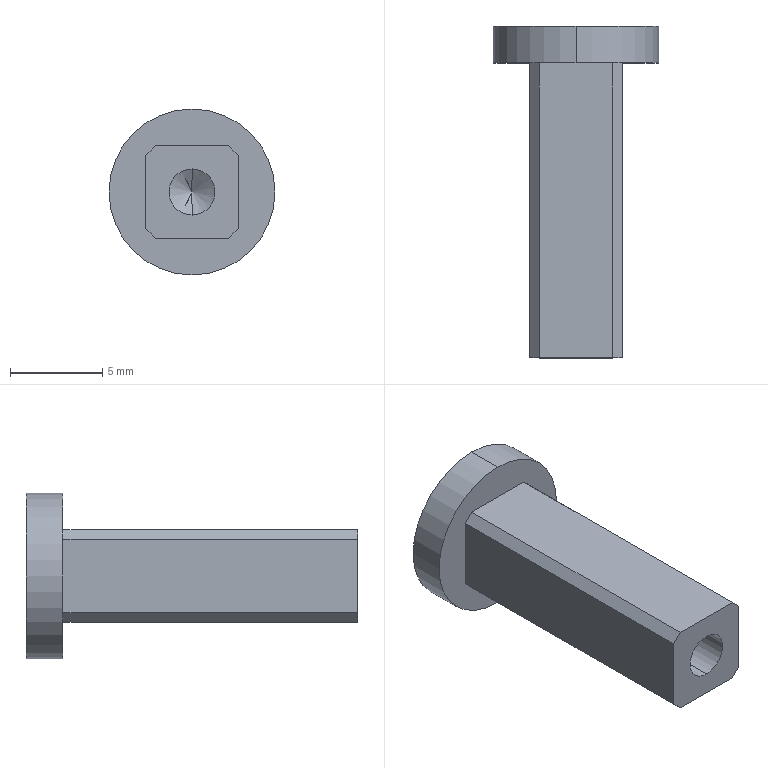Part | SolidWorks | features Chamfer 1, Extrusion 1, HoleWzd 1, ICE 1 | 1 solid | 17 faces | box 9 x 18 x 9 mm | volume 476.281 mm3 | plane 11 | cylinder 4 | cone 2 | commonest cylinder face diameters 2.5 x2 9 x2
STEP:
#1=CARTESIAN_POINT('',(0.,-0.5,1.25));
#2=VERTEX_POINT('',#1);
#3=CARTESIAN_POINT('',(0.,-0.5,-1.25));
#4=VERTEX_POINT('',#3);
#5=CARTESIAN_POINT('',(0.,-0.5,0.));
#6=DIRECTION('',(0.,-1.,0.));
#7=DIRECTION('',(0.,0.,-1.));
#8=AXIS2_PLACEMENT_3D('',#5,#6,#7);
#9=CIRCLE('',#8,1.25);
#10=EDGE_CURVE('',#2,#4,#9,.T.);
#11=ORIENTED_EDGE('',*,*,#10,.F.);
#12=CARTESIAN_POINT('',(0.,-9.,1.25));
#13=VERTEX_POINT('',#12);
#14=CARTESIAN_POINT('',(0.,-9.,1.25));
#15=DIRECTION('',(0.,-1.,0.));
#16=VECTOR('',#15,1000.);
#17=LINE('',#14,#16);
#18=EDGE_CURVE('',#2,#13,#17,.T.);
#19=ORIENTED_EDGE('',*,*,#18,.T.);
#20=CARTESIAN_POINT('',(0.,-9.,-1.25));
#21=VERTEX_POINT('',#20);
#22=CARTESIAN_POINT('',(0.,-9.,0.));
#23=DIRECTION('',(0.,-1.,0.));
#24=DIRECTION('',(0.,0.,-1.));
#25=AXIS2_PLACEMENT_3D('',#22,#23,#24);
#26=CIRCLE('',#25,1.25);
#27=EDGE_CURVE('',#13,#21,#26,.T.);
#28=ORIENTED_EDGE('',*,*,#27,.T.);
#29=CARTESIAN_POINT('',(0.,-9.,-1.25));
#30=DIRECTION('',(0.,-1.,0.));
#31=VECTOR('',#30,1000.);
#32=LINE('',#29,#31);
#33=EDGE_CURVE('',#4,#21,#32,.T.);
#34=ORIENTED_EDGE('',*,*,#33,.F.);
#35=EDGE_LOOP('',(#11,#19,#28,#34));
#36=FACE_OUTER_BOUND('',#35,.T.);
#37=CARTESIAN_POINT('',(0.,-9.,0.));
#38=DIRECTION('',(0.,-1.,0.));
#39=DIRECTION('',(0.,0.,-1.));
#40=AXIS2_PLACEMENT_3D('',#37,#38,#39);
#41=CYLINDRICAL_SURFACE('',#40,1.25);
#42=ADVANCED_FACE('',(#36),#41,.F.);
#43=CARTESIAN_POINT('',(0.,0.2511,0.));
#44=VERTEX_POINT('',#43);
#45=CARTESIAN_POINT('',(0.,-0.5,-1.25));
#46=DIRECTION('',(0.,-0.515,-0.8572));
#47=VECTOR('',#46,1000.);
#48=LINE('',#45,#47);
#49=EDGE_CURVE('',#44,#4,#48,.T.);
#50=ORIENTED_EDGE('',*,*,#49,.F.);
#51=CARTESIAN_POINT('',(0.,-0.5,1.25));
#52=DIRECTION('',(0.,-0.515,0.8572));
#53=VECTOR('',#52,1000.);
#54=LINE('',#51,#53);
#55=EDGE_CURVE('',#44,#2,#54,.T.);
#56=ORIENTED_EDGE('',*,*,#55,.T.);
#57=ORIENTED_EDGE('',*,*,#10,.T.);
#58=EDGE_LOOP('',(#50,#56,#57));
#59=FACE_OUTER_BOUND('',#58,.T.);
#60=CARTESIAN_POINT('',(0.,-0.5,0.));
#61=DIRECTION('',(0.,-1.,0.));
#62=DIRECTION('',(0.,0.,-1.));
#63=AXIS2_PLACEMENT_3D('',#60,#61,#62);
#64=CONICAL_SURFACE('',#63,1.25,1.03);
#65=ADVANCED_FACE('',(#59),#64,.F.);
#66=CARTESIAN_POINT('',(0.,9.,4.5));
#67=VERTEX_POINT('',#66);
#68=CARTESIAN_POINT('',(0.,9.,-4.5));
#69=VERTEX_POINT('',#68);
#70=CARTESIAN_POINT('',(0.,9.,0.));
#71=DIRECTION('',(0.,1.,0.));
#72=DIRECTION('',(0.,0.,1.));
#73=AXIS2_PLACEMENT_3D('',#70,#71,#72);
#74=CIRCLE('',#73,4.5);
#75=EDGE_CURVE('',#67,#69,#74,.T.);
#76=ORIENTED_EDGE('',*,*,#75,.F.);
#77=CARTESIAN_POINT('',(0.,7.,4.5));
#78=VERTEX_POINT('',#77);
#79=CARTESIAN_POINT('',(0.,9.,4.5));
#80=DIRECTION('',(0.,-1.,0.));
#81=VECTOR('',#80,1000.);
#82=LINE('',#79,#81);
#83=EDGE_CURVE('',#67,#78,#82,.T.);
#84=ORIENTED_EDGE('',*,*,#83,.T.);
#85=CARTESIAN_POINT('',(0.,7.,-4.5));
#86=VERTEX_POINT('',#85);
#87=CARTESIAN_POINT('',(0.,7.,0.));
#88=DIRECTION('',(0.,-1.,0.));
#89=DIRECTION('',(0.,0.,-1.));
#90=AXIS2_PLACEMENT_3D('',#87,#88,#89);
#91=CIRCLE('',#90,4.5);
#92=EDGE_CURVE('',#86,#78,#91,.T.);
#93=ORIENTED_EDGE('',*,*,#92,.F.);
#94=CARTESIAN_POINT('',(0.,9.,-4.5));
#95=DIRECTION('',(0.,-1.,0.));
#96=VECTOR('',#95,1000.);
#97=LINE('',#94,#96);
#98=EDGE_CURVE('',#69,#86,#97,.T.);
#99=ORIENTED_EDGE('',*,*,#98,.F.);
#100=EDGE_LOOP('',(#76,#84,#93,#99));
#101=FACE_OUTER_BOUND('',#100,.T.);
#102=CARTESIAN_POINT('',(0.,9.,0.));
#103=DIRECTION('',(0.,-1.,0.));
#104=DIRECTION('',(0.,0.,-1.));
#105=AXIS2_PLACEMENT_3D('',#102,#103,#104);
#106=CYLINDRICAL_SURFACE('',#105,4.5);
#107=ADVANCED_FACE('',(#101),#106,.T.);
#108=ORIENTED_EDGE('',*,*,#83,.F.);
#109=CARTESIAN_POINT('',(0.,9.,0.));
#110=DIRECTION('',(0.,1.,0.));
#111=DIRECTION('',(0.,0.,1.));
#112=AXIS2_PLACEMENT_3D('',#109,#110,#111);
#113=CIRCLE('',#112,4.5);
#114=EDGE_CURVE('',#69,#67,#113,.T.);
#115=ORIENTED_EDGE('',*,*,#114,.F.);
#116=ORIENTED_EDGE('',*,*,#98,.T.);
#117=CARTESIAN_POINT('',(0.,7.,0.));
#118=DIRECTION('',(0.,-1.,0.));
#119=DIRECTION('',(0.,0.,-1.));
#120=AXIS2_PLACEMENT_3D('',#117,#118,#119);
#121=CIRCLE('',#120,4.5);
#122=EDGE_CURVE('',#78,#86,#121,.T.);
#123=ORIENTED_EDGE('',*,*,#122,.F.);
#124=EDGE_LOOP('',(#108,#115,#116,#123));
#125=FACE_OUTER_BOUND('',#124,.T.);
#126=CARTESIAN_POINT('',(0.,9.,0.));
#127=DIRECTION('',(0.,-1.,0.));
#128=DIRECTION('',(0.,0.,-1.));
#129=AXIS2_PLACEMENT_3D('',#126,#127,#128);
#130=CYLINDRICAL_SURFACE('',#129,4.5);
#131=ADVANCED_FACE('',(#125),#130,.T.);
#132=ORIENTED_EDGE('',*,*,#114,.T.);
#133=ORIENTED_EDGE('',*,*,#75,.T.);
#134=EDGE_LOOP('',(#132,#133));
#135=FACE_OUTER_BOUND('',#134,.T.);
#136=CARTESIAN_POINT('',(0.,9.,0.));
#137=DIRECTION('',(0.,1.,0.));
#138=DIRECTION('',(0.,0.,1.));
#139=AXIS2_PLACEMENT_3D('',#136,#137,#138);
#140=PLANE('',#139);
#141=ADVANCED_FACE('',(#135),#140,.T.);
#142=CARTESIAN_POINT('',(-2.,7.,-2.5));
#143=VERTEX_POINT('',#142);
#144=CARTESIAN_POINT('',(2.,7.,-2.5));
#145=VERTEX_POINT('',#144);
#146=CARTESIAN_POINT('',(-2.5,7.,-2.5));
#147=DIRECTION('',(1.,0.,0.));
#148=VECTOR('',#147,1000.);
#149=LINE('',#146,#148);
#150=EDGE_CURVE('',#143,#145,#149,.T.);
#151=ORIENTED_EDGE('',*,*,#150,.F.);
#152=CARTESIAN_POINT('',(-2.5,7.,-2.));
#153=VERTEX_POINT('',#152);
#154=CARTESIAN_POINT('',(-2.5,7.,-2.));
#155=DIRECTION('',(-0.7071,0.,0.7071));
#156=VECTOR('',#155,1000.);
#157=LINE('',#154,#156);
#158=EDGE_CURVE('',#143,#153,#157,.T.);
#159=ORIENTED_EDGE('',*,*,#158,.T.);
#160=CARTESIAN_POINT('',(-2.5,7.,2.));
#161=VERTEX_POINT('',#160);
#162=CARTESIAN_POINT('',(-2.5,7.,-2.5));
#163=DIRECTION('',(0.,0.,-1.));
#164=VECTOR('',#163,1000.);
#165=LINE('',#162,#164);
#166=EDGE_CURVE('',#161,#153,#165,.T.);
#167=ORIENTED_EDGE('',*,*,#166,.F.);
#168=CARTESIAN_POINT('',(-2.,7.,2.5));
#169=VERTEX_POINT('',#168);
#170=CARTESIAN_POINT('',(-2.,7.,2.5));
#171=DIRECTION('',(0.7071,0.,0.7071));
#172=VECTOR('',#171,1000.);
#173=LINE('',#170,#172);
#174=EDGE_CURVE('',#161,#169,#173,.T.);
#175=ORIENTED_EDGE('',*,*,#174,.T.);
#176=CARTESIAN_POINT('',(2.,7.,2.5));
#177=VERTEX_POINT('',#176);
#178=CARTESIAN_POINT('',(-2.5,7.,2.5));
#179=DIRECTION('',(-1.,0.,0.));
#180=VECTOR('',#179,1000.);
#181=LINE('',#178,#180);
#182=EDGE_CURVE('',#177,#169,#181,.T.);
#183=ORIENTED_EDGE('',*,*,#182,.F.);
#184=CARTESIAN_POINT('',(2.5,7.,2.));
#185=VERTEX_POINT('',#184);
#186=CARTESIAN_POINT('',(2.5,7.,2.));
#187=DIRECTION('',(0.7071,0.,-0.7071));
#188=VECTOR('',#187,1000.);
#189=LINE('',#186,#188);
#190=EDGE_CURVE('',#177,#185,#189,.T.);
#191=ORIENTED_EDGE('',*,*,#190,.T.);
#192=CARTESIAN_POINT('',(2.5,7.,-2.));
#193=VERTEX_POINT('',#192);
#194=CARTESIAN_POINT('',(2.5,7.,-2.5));
#195=DIRECTION('',(0.,0.,1.));
#196=VECTOR('',#195,1000.);
#197=LINE('',#194,#196);
#198=EDGE_CURVE('',#193,#185,#197,.T.);
#199=ORIENTED_EDGE('',*,*,#198,.F.);
#200=CARTESIAN_POINT('',(2.,7.,-2.5));
#201=DIRECTION('',(-0.7071,0.,-0.7071));
#202=VECTOR('',#201,1000.);
#203=LINE('',#200,#202);
#204=EDGE_CURVE('',#193,#145,#203,.T.);
#205=ORIENTED_EDGE('',*,*,#204,.T.);
#206=EDGE_LOOP('',(#151,#159,#167,#175,#183,#191,#199,#205));
#207=FACE_BOUND('',#206,.T.);
#208=ORIENTED_EDGE('',*,*,#92,.T.);
#209=ORIENTED_EDGE('',*,*,#122,.T.);
#210=EDGE_LOOP('',(#208,#209));
#211=FACE_OUTER_BOUND('',#210,.T.);
#212=CARTESIAN_POINT('',(0.,7.,0.));
#213=DIRECTION('',(0.,-1.,0.));
#214=DIRECTION('',(0.,0.,-1.));
#215=AXIS2_PLACEMENT_3D('',#212,#213,#214);
#216=PLANE('',#215);
#217=ADVANCED_FACE('',(#207,#211),#216,.T.);
#218=CARTESIAN_POINT('',(2.5,-9.,-2.));
#219=VERTEX_POINT('',#218);
#220=CARTESIAN_POINT('',(2.5,-9.,2.));
#221=VERTEX_POINT('',#220);
#222=CARTESIAN_POINT('',(2.5,-9.,-2.5));
#223=DIRECTION('',(0.,0.,1.));
#224=VECTOR('',#223,1000.);
#225=LINE('',#222,#224);
#226=EDGE_CURVE('',#219,#221,#225,.T.);
#227=ORIENTED_EDGE('',*,*,#226,.F.);
#228=CARTESIAN_POINT('',(2.5,7.,-2.));
#229=DIRECTION('',(0.,1.,0.));
#230=VECTOR('',#229,1000.);
#231=LINE('',#228,#230);
#232=EDGE_CURVE('',#219,#193,#231,.T.);
#233=ORIENTED_EDGE('',*,*,#232,.T.);
#234=ORIENTED_EDGE('',*,*,#198,.T.);
#235=CARTESIAN_POINT('',(2.5,7.,2.));
#236=DIRECTION('',(0.,-1.,0.));
#237=VECTOR('',#236,1000.);
#238=LINE('',#235,#237);
#239=EDGE_CURVE('',#185,#221,#238,.T.);
#240=ORIENTED_EDGE('',*,*,#239,.T.);
#241=EDGE_LOOP('',(#227,#233,#234,#240));
#242=FACE_OUTER_BOUND('',#241,.T.);
#243=CARTESIAN_POINT('',(2.5,7.,-2.5));
#244=DIRECTION('',(1.,0.,0.));
#245=DIRECTION('',(0.,0.,-1.));
#246=AXIS2_PLACEMENT_3D('',#243,#244,#245);
#247=PLANE('',#246);
#248=ADVANCED_FACE('',(#242),#247,.T.);
#249=CARTESIAN_POINT('',(-2.,-9.,-2.5));
#250=VERTEX_POINT('',#249);
#251=CARTESIAN_POINT('',(2.,-9.,-2.5));
#252=VERTEX_POINT('',#251);
#253=CARTESIAN_POINT('',(-2.5,-9.,-2.5));
#254=DIRECTION('',(1.,0.,0.));
#255=VECTOR('',#254,1000.);
#256=LINE('',#253,#255);
#257=EDGE_CURVE('',#250,#252,#256,.T.);
#258=ORIENTED_EDGE('',*,*,#257,.F.);
#259=CARTESIAN_POINT('',(-2.,7.,-2.5));
#260=DIRECTION('',(0.,1.,0.));
#261=VECTOR('',#260,1000.);
#262=LINE('',#259,#261);
#263=EDGE_CURVE('',#250,#143,#262,.T.);
#264=ORIENTED_EDGE('',*,*,#263,.T.);
#265=ORIENTED_EDGE('',*,*,#150,.T.);
#266=CARTESIAN_POINT('',(2.,7.,-2.5));
#267=DIRECTION('',(0.,-1.,0.));
#268=VECTOR('',#267,1000.);
#269=LINE('',#266,#268);
#270=EDGE_CURVE('',#145,#252,#269,.T.);
#271=ORIENTED_EDGE('',*,*,#270,.T.);
#272=EDGE_LOOP('',(#258,#264,#265,#271));
#273=FACE_OUTER_BOUND('',#272,.T.);
#274=CARTESIAN_POINT('',(-2.5,7.,-2.5));
#275=DIRECTION('',(0.,0.,-1.));
#276=DIRECTION('',(-1.,0.,0.));
#277=AXIS2_PLACEMENT_3D('',#274,#275,#276);
#278=PLANE('',#277);
#279=ADVANCED_FACE('',(#273),#278,.T.);
#280=ORIENTED_EDGE('',*,*,#166,.T.);
#281=CARTESIAN_POINT('',(-2.5,-9.,-2.));
#282=VERTEX_POINT('',#281);
#283=CARTESIAN_POINT('',(-2.5,7.,-2.));
#284=DIRECTION('',(0.,-1.,0.));
#285=VECTOR('',#284,1000.);
#286=LINE('',#283,#285);
#287=EDGE_CURVE('',#153,#282,#286,.T.);
#288=ORIENTED_EDGE('',*,*,#287,.T.);
#289=CARTESIAN_POINT('',(-2.5,-9.,2.));
#290=VERTEX_POINT('',#289);
#291=CARTESIAN_POINT('',(-2.5,-9.,-2.5));
#292=DIRECTION('',(0.,0.,-1.));
#293=VECTOR('',#292,1000.);
#294=LINE('',#291,#293);
#295=EDGE_CURVE('',#290,#282,#294,.T.);
#296=ORIENTED_EDGE('',*,*,#295,.F.);
#297=CARTESIAN_POINT('',(-2.5,7.,2.));
#298=DIRECTION('',(0.,1.,0.));
#299=VECTOR('',#298,1000.);
#300=LINE('',#297,#299);
#301=EDGE_CURVE('',#290,#161,#300,.T.);
#302=ORIENTED_EDGE('',*,*,#301,.T.);
#303=EDGE_LOOP('',(#280,#288,#296,#302));
#304=FACE_OUTER_BOUND('',#303,.T.);
#305=CARTESIAN_POINT('',(-2.5,7.,-2.5));
#306=DIRECTION('',(-1.,0.,0.));
#307=DIRECTION('',(0.,0.,1.));
#308=AXIS2_PLACEMENT_3D('',#305,#306,#307);
#309=PLANE('',#308);
#310=ADVANCED_FACE('',(#304),#309,.T.);
#311=ORIENTED_EDGE('',*,*,#182,.T.);
#312=CARTESIAN_POINT('',(-2.,-9.,2.5));
#313=VERTEX_POINT('',#312);
#314=CARTESIAN_POINT('',(-2.,7.,2.5));
#315=DIRECTION('',(0.,-1.,0.));
#316=VECTOR('',#315,1000.);
#317=LINE('',#314,#316);
#318=EDGE_CURVE('',#169,#313,#317,.T.);
#319=ORIENTED_EDGE('',*,*,#318,.T.);
#320=CARTESIAN_POINT('',(2.,-9.,2.5));
#321=VERTEX_POINT('',#320);
#322=CARTESIAN_POINT('',(-2.5,-9.,2.5));
#323=DIRECTION('',(-1.,0.,0.));
#324=VECTOR('',#323,1000.);
#325=LINE('',#322,#324);
#326=EDGE_CURVE('',#321,#313,#325,.T.);
#327=ORIENTED_EDGE('',*,*,#326,.F.);
#328=CARTESIAN_POINT('',(2.,7.,2.5));
#329=DIRECTION('',(0.,1.,0.));
#330=VECTOR('',#329,1000.);
#331=LINE('',#328,#330);
#332=EDGE_CURVE('',#321,#177,#331,.T.);
#333=ORIENTED_EDGE('',*,*,#332,.T.);
#334=EDGE_LOOP('',(#311,#319,#327,#333));
#335=FACE_OUTER_BOUND('',#334,.T.);
#336=CARTESIAN_POINT('',(-2.5,7.,2.5));
#337=DIRECTION('',(0.,0.,1.));
#338=DIRECTION('',(1.,0.,0.));
#339=AXIS2_PLACEMENT_3D('',#336,#337,#338);
#340=PLANE('',#339);
#341=ADVANCED_FACE('',(#335),#340,.T.);
#342=CARTESIAN_POINT('',(0.,-9.,0.));
#343=DIRECTION('',(0.,-1.,0.));
#344=DIRECTION('',(0.,0.,-1.));
#345=AXIS2_PLACEMENT_3D('',#342,#343,#344);
#346=CIRCLE('',#345,1.25);
#347=EDGE_CURVE('',#21,#13,#346,.T.);
#348=ORIENTED_EDGE('',*,*,#347,.F.);
#349=ORIENTED_EDGE('',*,*,#27,.F.);
#350=EDGE_LOOP('',(#348,#349));
#351=FACE_BOUND('',#350,.T.);
#352=ORIENTED_EDGE('',*,*,#295,.T.);
#353=CARTESIAN_POINT('',(-2.5,-9.,-2.));
#354=DIRECTION('',(0.7071,0.,-0.7071));
#355=VECTOR('',#354,1000.);
#356=LINE('',#353,#355);
#357=EDGE_CURVE('',#282,#250,#356,.T.);
#358=ORIENTED_EDGE('',*,*,#357,.T.);
#359=ORIENTED_EDGE('',*,*,#257,.T.);
#360=CARTESIAN_POINT('',(2.,-9.,-2.5));
#361=DIRECTION('',(0.7071,0.,0.7071));
#362=VECTOR('',#361,1000.);
#363=LINE('',#360,#362);
#364=EDGE_CURVE('',#252,#219,#363,.T.);
#365=ORIENTED_EDGE('',*,*,#364,.T.);
#366=ORIENTED_EDGE('',*,*,#226,.T.);
#367=CARTESIAN_POINT('',(2.5,-9.,2.));
#368=DIRECTION('',(-0.7071,0.,0.7071));
#369=VECTOR('',#368,1000.);
#370=LINE('',#367,#369);
#371=EDGE_CURVE('',#221,#321,#370,.T.);
#372=ORIENTED_EDGE('',*,*,#371,.T.);
#373=ORIENTED_EDGE('',*,*,#326,.T.);
#374=CARTESIAN_POINT('',(-2.,-9.,2.5));
#375=DIRECTION('',(-0.7071,0.,-0.7071));
#376=VECTOR('',#375,1000.);
#377=LINE('',#374,#376);
#378=EDGE_CURVE('',#313,#290,#377,.T.);
#379=ORIENTED_EDGE('',*,*,#378,.T.);
#380=EDGE_LOOP('',(#352,#358,#359,#365,#366,#372,#373,#379));
#381=FACE_OUTER_BOUND('',#380,.T.);
#382=CARTESIAN_POINT('',(0.,-9.,0.));
#383=DIRECTION('',(0.,1.,0.));
#384=DIRECTION('',(0.,0.,1.));
#385=AXIS2_PLACEMENT_3D('',#382,#383,#384);
#386=PLANE('',#385);
#387=ADVANCED_FACE('',(#351,#381),#386,.F.);
#388=ORIENTED_EDGE('',*,*,#55,.F.);
#389=ORIENTED_EDGE('',*,*,#49,.T.);
#390=CARTESIAN_POINT('',(0.,-0.5,0.));
#391=DIRECTION('',(0.,-1.,0.));
#392=DIRECTION('',(0.,0.,-1.));
#393=AXIS2_PLACEMENT_3D('',#390,#391,#392);
#394=CIRCLE('',#393,1.25);
#395=EDGE_CURVE('',#4,#2,#394,.T.);
#396=ORIENTED_EDGE('',*,*,#395,.T.);
#397=EDGE_LOOP('',(#388,#389,#396));
#398=FACE_OUTER_BOUND('',#397,.T.);
#399=CARTESIAN_POINT('',(0.,-0.5,0.));
#400=DIRECTION('',(0.,-1.,0.));
#401=DIRECTION('',(0.,0.,-1.));
#402=AXIS2_PLACEMENT_3D('',#399,#400,#401);
#403=CONICAL_SURFACE('',#402,1.25,1.03);
#404=ADVANCED_FACE('',(#398),#403,.F.);
#405=ORIENTED_EDGE('',*,*,#18,.F.);
#406=ORIENTED_EDGE('',*,*,#395,.F.);
#407=ORIENTED_EDGE('',*,*,#33,.T.);
#408=ORIENTED_EDGE('',*,*,#347,.T.);
#409=EDGE_LOOP('',(#405,#406,#407,#408));
#410=FACE_OUTER_BOUND('',#409,.T.);
#411=CARTESIAN_POINT('',(0.,-9.,0.));
#412=DIRECTION('',(0.,-1.,0.));
#413=DIRECTION('',(0.,0.,-1.));
#414=AXIS2_PLACEMENT_3D('',#411,#412,#413);
#415=CYLINDRICAL_SURFACE('',#414,1.25);
#416=ADVANCED_FACE('',(#410),#415,.F.);
#417=ORIENTED_EDGE('',*,*,#158,.F.);
#418=ORIENTED_EDGE('',*,*,#263,.F.);
#419=ORIENTED_EDGE('',*,*,#357,.F.);
#420=ORIENTED_EDGE('',*,*,#287,.F.);
#421=EDGE_LOOP('',(#417,#418,#419,#420));
#422=FACE_OUTER_BOUND('',#421,.T.);
#423=CARTESIAN_POINT('',(-2.5,7.,-2.));
#424=DIRECTION('',(0.7071,0.,0.7071));
#425=DIRECTION('',(0.,-1.,0.));
#426=AXIS2_PLACEMENT_3D('',#423,#424,#425);
#427=PLANE('',#426);
#428=ADVANCED_FACE('',(#422),#427,.F.);
#429=ORIENTED_EDGE('',*,*,#204,.F.);
#430=ORIENTED_EDGE('',*,*,#232,.F.);
#431=ORIENTED_EDGE('',*,*,#364,.F.);
#432=ORIENTED_EDGE('',*,*,#270,.F.);
#433=EDGE_LOOP('',(#429,#430,#431,#432));
#434=FACE_OUTER_BOUND('',#433,.T.);
#435=CARTESIAN_POINT('',(2.,7.,-2.5));
#436=DIRECTION('',(-0.7071,0.,0.7071));
#437=DIRECTION('',(0.,-1.,0.));
#438=AXIS2_PLACEMENT_3D('',#435,#436,#437);
#439=PLANE('',#438);
#440=ADVANCED_FACE('',(#434),#439,.F.);
#441=ORIENTED_EDGE('',*,*,#174,.F.);
#442=ORIENTED_EDGE('',*,*,#301,.F.);
#443=ORIENTED_EDGE('',*,*,#378,.F.);
#444=ORIENTED_EDGE('',*,*,#318,.F.);
#445=EDGE_LOOP('',(#441,#442,#443,#444));
#446=FACE_OUTER_BOUND('',#445,.T.);
#447=CARTESIAN_POINT('',(-2.,7.,2.5));
#448=DIRECTION('',(0.7071,0.,-0.7071));
#449=DIRECTION('',(0.,-1.,0.));
#450=AXIS2_PLACEMENT_3D('',#447,#448,#449);
#451=PLANE('',#450);
#452=ADVANCED_FACE('',(#446),#451,.F.);
#453=ORIENTED_EDGE('',*,*,#190,.F.);
#454=ORIENTED_EDGE('',*,*,#332,.F.);
#455=ORIENTED_EDGE('',*,*,#371,.F.);
#456=ORIENTED_EDGE('',*,*,#239,.F.);
#457=EDGE_LOOP('',(#453,#454,#455,#456));
#458=FACE_OUTER_BOUND('',#457,.T.);
#459=CARTESIAN_POINT('',(2.5,7.,2.));
#460=DIRECTION('',(-0.7071,0.,-0.7071));
#461=DIRECTION('',(0.,-1.,0.));
#462=AXIS2_PLACEMENT_3D('',#459,#460,#461);
#463=PLANE('',#462);
#464=ADVANCED_FACE('',(#458),#463,.F.);
#465=CLOSED_SHELL('',(#42,#65,#107,#131,#141,#217,#248,#279,#310,#341,#387,#404,#416,#428,#440,#452,#464));
#466=MANIFOLD_SOLID_BREP('',#465);
#467=CARTESIAN_POINT('',(0.,0.,0.));
#468=DIRECTION('',(0.,0.,1.));
#469=DIRECTION('',(1.,0.,0.));
#470=AXIS2_PLACEMENT_3D('',#467,#468,#469);
#471=(LENGTH_UNIT()NAMED_UNIT(*)SI_UNIT(.MILLI.,.METRE.));
#472=UNCERTAINTY_MEASURE_WITH_UNIT(LENGTH_MEASURE(0.00001),#471,'','');
#473=(NAMED_UNIT(*)PLANE_ANGLE_UNIT()SI_UNIT($,.RADIAN.));
#474=(NAMED_UNIT(*)SI_UNIT($,.STERADIAN.)SOLID_ANGLE_UNIT());
#475=(GEOMETRIC_REPRESENTATION_CONTEXT(3)GLOBAL_UNCERTAINTY_ASSIGNED_CONTEXT((#472))GLOBAL_UNIT_ASSIGNED_CONTEXT((#471,#473,#474))REPRESENTATION_CONTEXT('',''));
#476=ADVANCED_BREP_SHAPE_REPRESENTATION('',(#466,#470),#475);